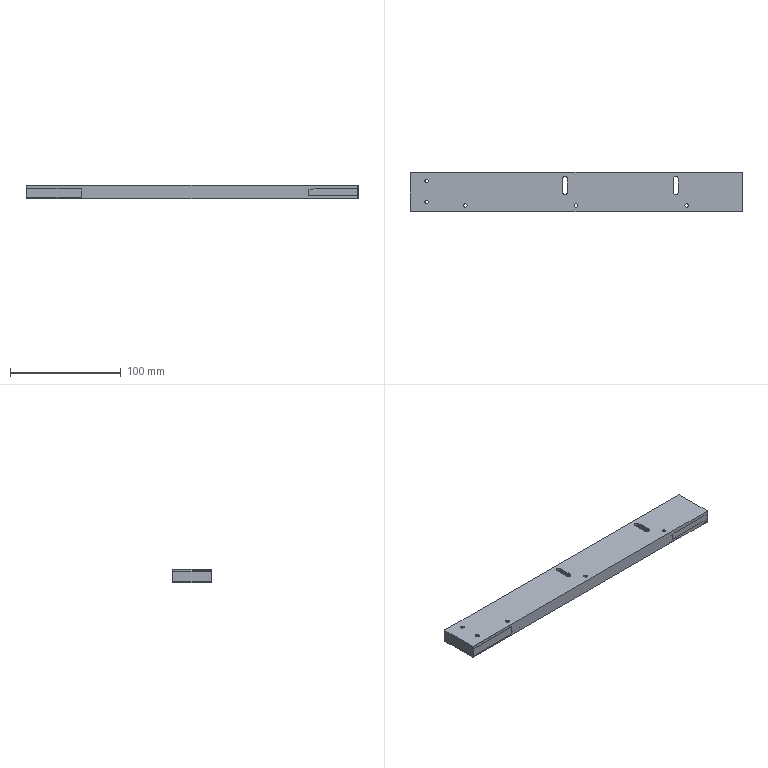CAM job | NX | 3+2 milling, drilling | part box 300 x 36 x 12 mm | stock box 305 x 41 x 15 mm
Tools:
number,name,description,diameter,corner_radius,flute_length,length,flutes
4,D4,平底铣刀-粗,4.0,0.0,25.0,75.0,2
6,D6,平底铣刀-粗,6.0,0.0,25.0,75.0,2
9,D10,平底铣刀-粗,10.0,0.0,35.0,75.0,2
11,D4-J,平底铣刀-精,4.0,0.0,50.0,75.0,2
7,D6-J,平底铣刀-精,6.0,0.0,25.0,75.0,2
10,D10-J,平底铣刀-精,10.0,0.0,35.0,75.0,2
2,D6倒角刀,倒角刀,6.0,0.0,3.0,25.0,2
21,M4X0.7,丝锥,3.3,0.0,35.0,50.0,2
13,ZT3.3,钻头,3.3,0.0,35.0,50.0,2
Operations:
program,operation,operation_type,tool,method,geometry_group,spindle_rpm,surface_speed,feed_per_tooth,feed_cut,feed_plunge,cut_length_mm,path_length_mm,cut_time_min,machine_time_min
E,底壁铣分层开粗-中_COPY,VolumeBased25DMillingOperation,D6,分层开粗-切深K-步距G,W-E,8000.0,150.792,0.1875,3000.0,100.0,2061.992,2080.974,0.6873,0.6892
E,底壁铣精光底面-中_COPY,VolumeBased25DMillingOperation,D6-J,精光步距切深关,W-E,8000.0,150.792,0.0625,1000.0,100.0,803.902,823.302,0.8039,0.8058
E,底壁铣精光侧面-中-选底面_COPY,VolumeBased25DMillingOperation,D6-J,侧刃精光-切深K-步距G,W-E,8000.0,150.792,0.0625,1000.0,100.0,145.884,359.084,0.1459,0.1672
E,等高精光往复爬面_COPY,ZLevelMilling,D6-J,等高爬面-切深K-步距G,W-E,8000.0,150.796,0.25,4000.0,100.0,23912.852,23939.299,5.978,5.981
E,等高精光往复爬面_COPY_COPY,ZLevelMilling,D6-J,等高爬面-切深K-步距G,W-E,8000.0,150.796,0.25,4000.0,100.0,6077.635,6098.193,1.519,1.522
E,等高精光往复爬面_COPY_COPY_COPY,ZLevelMilling,D6-J,等高爬面-切深K-步距G,W-E,8000.0,150.796,0.25,4000.0,100.0,4221.597,4243.594,1.055,1.058
D,面铣自动飞面精光_COPY_COPY_COPY_1_COPY,FaceMilling,D10-J,侧刃精光-切深K-步距G,W-D,8000.0,251.327,0.0625,1000.0,100.0,4820.633,5221.609,4.821,4.861
D,面铣自动飞面精光_COPY_COPY_COPY_1_COPY_COPY,FaceMilling,D10-J,侧刃精光-切深K-步距G,W-D,8000.0,251.327,0.0625,1000.0,100.0,2410.317,2506.317,2.41,2.42
D,底壁铣分层开粗-中_COPY_2,VolumeBased25DMillingOperation,D6,分层开粗-切深K-步距G,W-D,8000.0,150.792,0.1875,3000.0,100.0,4659.925,5305.181,1.553,1.618
D,打点-深0.8,Operation,D6倒角刀,NONE,W-D,8000.0,150.796,0.0312,500.0,90.0,9.0,377.497,0.018,0.0548
D,通孔-M4螺纹底孔,Operation,ZT3.3,NONE,W-D,3000.0,30.536,0.05,300.0,90.0,85.0,529.497,0.2833,0.3278
D,钻倒角_2,Operation,D6倒角刀,METHOD,W-D,8000.0,150.796,0.0312,500.0,0.0,25.855,419.732,0.0517,0.0911
D,通孔-攻牙M4,Operation,M4X0.7,METHOD,W-D,600.0,6.22,0.0006,0.7,90.0,70.0,498.197,100.0,100.043
D,底壁铣倒角_COPY,VolumeBased25DMillingOperation,D6倒角刀,爬面_倒角-切深0-步距G,W-D,6500.0,122.519,0.1154,1500.0,100.0,349.496,448.896,0.233,0.2429
D,平面去毛刺6X45L_COPY,SurfaceContour,D6倒角刀,爬面_倒角-切深0-步距G,W-D,6500.0,122.519,0.1154,1500.0,100.0,754.625,2044.88,0.5031,0.6321
D,底壁铣精光底面-中_COPY_2,VolumeBased25DMillingOperation,D6-J,精光步距切深关,W-D,8000.0,150.792,0.0625,1000.0,100.0,1838.276,1859.676,1.838,1.84
D,底壁铣精光侧面-中-选底面_COPY_3,VolumeBased25DMillingOperation,D6-J,侧刃精光-切深K-步距G,W-D,8000.0,150.792,0.0625,1000.0,100.0,312.168,334.568,0.3122,0.3144
C,面铣自动飞面精光_COPY_COPY_COPY,FaceMilling,D10-J,侧刃精光-切深K-步距G,W-C,8000.0,251.327,0.0625,1000.0,100.0,4820.633,5253.341,4.821,4.864
C,面铣自动飞面精光_COPY_COPY_1,FaceMilling,D10-J,侧刃精光-切深K-步距G,W-C,8000.0,251.327,0.0625,1000.0,100.0,2410.317,2506.317,2.41,2.42
C,通腰槽粗_1,VolumeBased25DMillingOperation,D4,METHOD,W-C,10000.0,125.664,0.06,1200.0,100.0,2247.933,2565.635,1.873,1.905
C,腰槽精_1,VolumeBased25DMillingOperation,D4-J,METHOD,W-C,8000.0,100.531,0.0312,500.0,100.0,166.795,542.399,0.3336,0.3711
C,钻倒角_1,Operation,D6倒角刀,METHOD,W-C,8000.0,150.796,0.0625,1000.0,0.0,25.855,418.309,0.0259,0.0651
C,C0.3封闭铣廓倒角6X45L_COPY_1,PlanarMilling,D6倒角刀,爬面_倒角-切深0-步距G,W-C,7000.0,131.0,0.1071,1500.0,100.0,781.992,1442.353,0.5213,0.5874
B,面铣自动飞面精光_COPY,FaceMilling,D10-J,侧刃精光-切深K-步距G,W-B,8000.0,251.327,0.0625,1000.0,100.0,12051.583,13495.253,12.052,12.196
B,面铣自动飞面精光_COPY_COPY,FaceMilling,D10-J,侧刃精光-切深K-步距G,W-B,8000.0,251.327,0.0625,1000.0,100.0,2410.317,2506.317,2.41,2.42
B,C0.3封闭铣廓倒角6X45L_COPY,PlanarMilling,D6倒角刀,爬面_倒角-切深0-步距G,W-B,7000.0,131.0,0.1071,1500.0,100.0,688.357,784.357,0.4589,0.4685
A,顶面_1,FaceMilling,D10-J,侧刃精光-切深K-步距G,W-A,4500.0,1385.0,0.1667,1500.0,100.0,2390.518,2486.518,1.594,1.603
A,外形粗_2,VolumeBased25DMillingOperation,D10,METHOD,W-A,8000.0,251.327,0.375,6000.0,80.0,11950.342,12060.842,1.992,2.003
A,仅选体,SurfaceContour,D6倒角刀,METHOD,W-A,8000.0,150.796,0.1875,3000.0,100.0,688.13,783.931,0.2294,0.239
A,外形半精_2,VolumeBased25DMillingOperation,D10-J,METHOD,W-A,9000.0,169.646,0.0667,1200.0,100.0,707.202,830.202,0.5893,0.6016